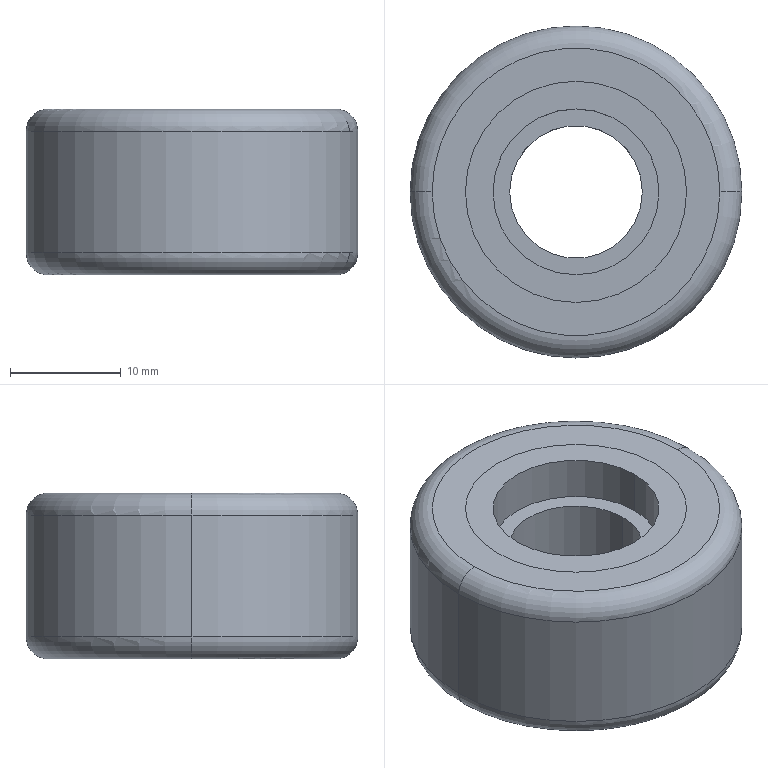Part | SolidWorks | features ICE 4, Extrusion 1, Fillet 1 | 2 solids | 22 faces | box 30 x 30 x 15 mm | volume 8240 mm3 | cylinder 12 | plane 6 | torus 4 | commonest cylinder face diameters 15 x4 20 x4 12 x2 30 x2
STEP:
#1=CARTESIAN_POINT('',(-15.,0.,13.));
#2=VERTEX_POINT('',#1);
#3=CARTESIAN_POINT('',(15.,0.,13.));
#4=VERTEX_POINT('',#3);
#5=CARTESIAN_POINT('',(0.,0.,13.));
#6=DIRECTION('',(0.,0.,-1.));
#7=DIRECTION('',(1.,0.,0.));
#8=AXIS2_PLACEMENT_3D('',#5,#6,#7);
#9=CIRCLE('',#8,15.);
#10=EDGE_CURVE('',#2,#4,#9,.T.);
#11=ORIENTED_EDGE('',*,*,#10,.F.);
#12=CARTESIAN_POINT('',(-13.,0.,15.));
#13=VERTEX_POINT('',#12);
#14=CARTESIAN_POINT('',(-13.,0.,13.));
#15=DIRECTION('',(0.,1.,0.));
#16=DIRECTION('',(-1.,0.,0.));
#17=AXIS2_PLACEMENT_3D('',#14,#15,#16);
#18=CIRCLE('',#17,2.);
#19=EDGE_CURVE('',#2,#13,#18,.T.);
#20=ORIENTED_EDGE('',*,*,#19,.T.);
#21=CARTESIAN_POINT('',(13.,0.,15.));
#22=VERTEX_POINT('',#21);
#23=CARTESIAN_POINT('',(0.,0.,15.));
#24=DIRECTION('',(0.,0.,1.));
#25=DIRECTION('',(1.,0.,0.));
#26=AXIS2_PLACEMENT_3D('',#23,#24,#25);
#27=CIRCLE('',#26,13.);
#28=EDGE_CURVE('',#22,#13,#27,.T.);
#29=ORIENTED_EDGE('',*,*,#28,.F.);
#30=CARTESIAN_POINT('',(13.,0.,13.));
#31=DIRECTION('',(0.,-1.,0.));
#32=DIRECTION('',(0.,0.,-1.));
#33=AXIS2_PLACEMENT_3D('',#30,#31,#32);
#34=CIRCLE('',#33,2.);
#35=EDGE_CURVE('',#4,#22,#34,.T.);
#36=ORIENTED_EDGE('',*,*,#35,.F.);
#37=EDGE_LOOP('',(#11,#20,#29,#36));
#38=FACE_OUTER_BOUND('',#37,.T.);
#39=CARTESIAN_POINT('',(0.,0.,13.));
#40=DIRECTION('',(0.,0.,1.));
#41=DIRECTION('',(1.,0.,0.));
#42=AXIS2_PLACEMENT_3D('',#39,#40,#41);
#43=TOROIDAL_SURFACE('',#42,13.,2.);
#44=ADVANCED_FACE('',(#38),#43,.T.);
#45=CARTESIAN_POINT('',(-13.,0.,0.));
#46=VERTEX_POINT('',#45);
#47=CARTESIAN_POINT('',(13.,0.,0.));
#48=VERTEX_POINT('',#47);
#49=CARTESIAN_POINT('',(0.,0.,0.));
#50=DIRECTION('',(0.,0.,-1.));
#51=DIRECTION('',(1.,0.,0.));
#52=AXIS2_PLACEMENT_3D('',#49,#50,#51);
#53=CIRCLE('',#52,13.);
#54=EDGE_CURVE('',#46,#48,#53,.T.);
#55=ORIENTED_EDGE('',*,*,#54,.F.);
#56=CARTESIAN_POINT('',(-15.,0.,2.));
#57=VERTEX_POINT('',#56);
#58=CARTESIAN_POINT('',(-13.,0.,2.));
#59=DIRECTION('',(0.,1.,0.));
#60=DIRECTION('',(-1.,0.,0.));
#61=AXIS2_PLACEMENT_3D('',#58,#59,#60);
#62=CIRCLE('',#61,2.);
#63=EDGE_CURVE('',#46,#57,#62,.T.);
#64=ORIENTED_EDGE('',*,*,#63,.T.);
#65=CARTESIAN_POINT('',(15.,0.,2.));
#66=VERTEX_POINT('',#65);
#67=CARTESIAN_POINT('',(0.,0.,2.));
#68=DIRECTION('',(0.,0.,1.));
#69=DIRECTION('',(1.,0.,0.));
#70=AXIS2_PLACEMENT_3D('',#67,#68,#69);
#71=CIRCLE('',#70,15.);
#72=EDGE_CURVE('',#66,#57,#71,.T.);
#73=ORIENTED_EDGE('',*,*,#72,.F.);
#74=CARTESIAN_POINT('',(13.,0.,2.));
#75=DIRECTION('',(0.,-1.,0.));
#76=DIRECTION('',(0.,0.,-1.));
#77=AXIS2_PLACEMENT_3D('',#74,#75,#76);
#78=CIRCLE('',#77,2.);
#79=EDGE_CURVE('',#48,#66,#78,.T.);
#80=ORIENTED_EDGE('',*,*,#79,.F.);
#81=EDGE_LOOP('',(#55,#64,#73,#80));
#82=FACE_OUTER_BOUND('',#81,.T.);
#83=CARTESIAN_POINT('',(0.,0.,2.));
#84=DIRECTION('',(0.,0.,1.));
#85=DIRECTION('',(1.,0.,0.));
#86=AXIS2_PLACEMENT_3D('',#83,#84,#85);
#87=TOROIDAL_SURFACE('',#86,13.,2.);
#88=ADVANCED_FACE('',(#82),#87,.T.);
#89=CARTESIAN_POINT('',(10.,0.,0.));
#90=VERTEX_POINT('',#89);
#91=CARTESIAN_POINT('',(-10.,0.,0.));
#92=VERTEX_POINT('',#91);
#93=CARTESIAN_POINT('',(0.,0.,0.));
#94=DIRECTION('',(0.,0.,-1.));
#95=DIRECTION('',(1.,0.,0.));
#96=AXIS2_PLACEMENT_3D('',#93,#94,#95);
#97=CIRCLE('',#96,10.);
#98=EDGE_CURVE('',#90,#92,#97,.T.);
#99=ORIENTED_EDGE('',*,*,#98,.T.);
#100=CARTESIAN_POINT('',(-10.,0.,15.));
#101=VERTEX_POINT('',#100);
#102=CARTESIAN_POINT('',(-10.,0.,-42.426));
#103=DIRECTION('',(0.,0.,1.));
#104=VECTOR('',#103,1000.);
#105=LINE('',#102,#104);
#106=EDGE_CURVE('',#92,#101,#105,.T.);
#107=ORIENTED_EDGE('',*,*,#106,.T.);
#108=CARTESIAN_POINT('',(10.,0.,15.));
#109=VERTEX_POINT('',#108);
#110=CARTESIAN_POINT('',(0.,0.,15.));
#111=DIRECTION('',(0.,0.,1.));
#112=DIRECTION('',(1.,0.,0.));
#113=AXIS2_PLACEMENT_3D('',#110,#111,#112);
#114=CIRCLE('',#113,10.);
#115=EDGE_CURVE('',#101,#109,#114,.T.);
#116=ORIENTED_EDGE('',*,*,#115,.T.);
#117=CARTESIAN_POINT('',(10.,0.,-42.426));
#118=DIRECTION('',(0.,0.,1.));
#119=VECTOR('',#118,1000.);
#120=LINE('',#117,#119);
#121=EDGE_CURVE('',#90,#109,#120,.T.);
#122=ORIENTED_EDGE('',*,*,#121,.F.);
#123=EDGE_LOOP('',(#99,#107,#116,#122));
#124=FACE_OUTER_BOUND('',#123,.T.);
#125=CARTESIAN_POINT('',(0.,0.,-42.426));
#126=DIRECTION('',(0.,0.,1.));
#127=DIRECTION('',(1.,0.,0.));
#128=AXIS2_PLACEMENT_3D('',#125,#126,#127);
#129=CYLINDRICAL_SURFACE('',#128,10.);
#130=ADVANCED_FACE('',(#124),#129,.F.);
#131=ORIENTED_EDGE('',*,*,#72,.T.);
#132=CARTESIAN_POINT('',(-15.,0.,-42.426));
#133=DIRECTION('',(0.,0.,1.));
#134=VECTOR('',#133,1000.);
#135=LINE('',#132,#134);
#136=EDGE_CURVE('',#57,#2,#135,.T.);
#137=ORIENTED_EDGE('',*,*,#136,.T.);
#138=ORIENTED_EDGE('',*,*,#10,.T.);
#139=CARTESIAN_POINT('',(15.,0.,-42.426));
#140=DIRECTION('',(0.,0.,1.));
#141=VECTOR('',#140,1000.);
#142=LINE('',#139,#141);
#143=EDGE_CURVE('',#66,#4,#142,.T.);
#144=ORIENTED_EDGE('',*,*,#143,.F.);
#145=EDGE_LOOP('',(#131,#137,#138,#144));
#146=FACE_OUTER_BOUND('',#145,.T.);
#147=CARTESIAN_POINT('',(0.,0.,-42.426));
#148=DIRECTION('',(0.,0.,1.));
#149=DIRECTION('',(1.,0.,0.));
#150=AXIS2_PLACEMENT_3D('',#147,#148,#149);
#151=CYLINDRICAL_SURFACE('',#150,15.);
#152=ADVANCED_FACE('',(#146),#151,.T.);
#153=ORIENTED_EDGE('',*,*,#136,.F.);
#154=CARTESIAN_POINT('',(0.,0.,2.));
#155=DIRECTION('',(0.,0.,1.));
#156=DIRECTION('',(1.,0.,0.));
#157=AXIS2_PLACEMENT_3D('',#154,#155,#156);
#158=CIRCLE('',#157,15.);
#159=EDGE_CURVE('',#57,#66,#158,.T.);
#160=ORIENTED_EDGE('',*,*,#159,.T.);
#161=ORIENTED_EDGE('',*,*,#143,.T.);
#162=CARTESIAN_POINT('',(0.,0.,13.));
#163=DIRECTION('',(0.,0.,-1.));
#164=DIRECTION('',(1.,0.,0.));
#165=AXIS2_PLACEMENT_3D('',#162,#163,#164);
#166=CIRCLE('',#165,15.);
#167=EDGE_CURVE('',#4,#2,#166,.T.);
#168=ORIENTED_EDGE('',*,*,#167,.T.);
#169=EDGE_LOOP('',(#153,#160,#161,#168));
#170=FACE_OUTER_BOUND('',#169,.T.);
#171=CARTESIAN_POINT('',(0.,0.,-42.426));
#172=DIRECTION('',(0.,0.,1.));
#173=DIRECTION('',(1.,0.,0.));
#174=AXIS2_PLACEMENT_3D('',#171,#172,#173);
#175=CYLINDRICAL_SURFACE('',#174,15.);
#176=ADVANCED_FACE('',(#170),#175,.T.);
#177=ORIENTED_EDGE('',*,*,#28,.T.);
#178=CARTESIAN_POINT('',(0.,0.,15.));
#179=DIRECTION('',(0.,0.,1.));
#180=DIRECTION('',(1.,0.,0.));
#181=AXIS2_PLACEMENT_3D('',#178,#179,#180);
#182=CIRCLE('',#181,13.);
#183=EDGE_CURVE('',#13,#22,#182,.T.);
#184=ORIENTED_EDGE('',*,*,#183,.T.);
#185=EDGE_LOOP('',(#177,#184));
#186=FACE_OUTER_BOUND('',#185,.T.);
#187=CARTESIAN_POINT('',(0.,0.,15.));
#188=DIRECTION('',(0.,0.,1.));
#189=DIRECTION('',(1.,0.,0.));
#190=AXIS2_PLACEMENT_3D('',#187,#188,#189);
#191=CIRCLE('',#190,10.);
#192=EDGE_CURVE('',#109,#101,#191,.T.);
#193=ORIENTED_EDGE('',*,*,#192,.F.);
#194=ORIENTED_EDGE('',*,*,#115,.F.);
#195=EDGE_LOOP('',(#193,#194));
#196=FACE_BOUND('',#195,.T.);
#197=CARTESIAN_POINT('',(0.,0.,15.));
#198=DIRECTION('',(0.,0.,1.));
#199=DIRECTION('',(1.,0.,0.));
#200=AXIS2_PLACEMENT_3D('',#197,#198,#199);
#201=PLANE('',#200);
#202=ADVANCED_FACE('',(#186,#196),#201,.T.);
#203=ORIENTED_EDGE('',*,*,#106,.F.);
#204=CARTESIAN_POINT('',(0.,0.,0.));
#205=DIRECTION('',(0.,0.,-1.));
#206=DIRECTION('',(1.,0.,0.));
#207=AXIS2_PLACEMENT_3D('',#204,#205,#206);
#208=CIRCLE('',#207,10.);
#209=EDGE_CURVE('',#92,#90,#208,.T.);
#210=ORIENTED_EDGE('',*,*,#209,.T.);
#211=ORIENTED_EDGE('',*,*,#121,.T.);
#212=ORIENTED_EDGE('',*,*,#192,.T.);
#213=EDGE_LOOP('',(#203,#210,#211,#212));
#214=FACE_OUTER_BOUND('',#213,.T.);
#215=CARTESIAN_POINT('',(0.,0.,-42.426));
#216=DIRECTION('',(0.,0.,1.));
#217=DIRECTION('',(1.,0.,0.));
#218=AXIS2_PLACEMENT_3D('',#215,#216,#217);
#219=CYLINDRICAL_SURFACE('',#218,10.);
#220=ADVANCED_FACE('',(#214),#219,.F.);
#221=CARTESIAN_POINT('',(0.,0.,0.));
#222=DIRECTION('',(0.,0.,-1.));
#223=DIRECTION('',(1.,0.,0.));
#224=AXIS2_PLACEMENT_3D('',#221,#222,#223);
#225=CIRCLE('',#224,13.);
#226=EDGE_CURVE('',#48,#46,#225,.T.);
#227=ORIENTED_EDGE('',*,*,#226,.T.);
#228=ORIENTED_EDGE('',*,*,#54,.T.);
#229=EDGE_LOOP('',(#227,#228));
#230=FACE_OUTER_BOUND('',#229,.T.);
#231=ORIENTED_EDGE('',*,*,#98,.F.);
#232=ORIENTED_EDGE('',*,*,#209,.F.);
#233=EDGE_LOOP('',(#231,#232));
#234=FACE_BOUND('',#233,.T.);
#235=CARTESIAN_POINT('',(0.,0.,0.));
#236=DIRECTION('',(0.,0.,1.));
#237=DIRECTION('',(1.,0.,0.));
#238=AXIS2_PLACEMENT_3D('',#235,#236,#237);
#239=PLANE('',#238);
#240=ADVANCED_FACE('',(#230,#234),#239,.F.);
#241=ORIENTED_EDGE('',*,*,#63,.F.);
#242=ORIENTED_EDGE('',*,*,#226,.F.);
#243=ORIENTED_EDGE('',*,*,#79,.T.);
#244=ORIENTED_EDGE('',*,*,#159,.F.);
#245=EDGE_LOOP('',(#241,#242,#243,#244));
#246=FACE_OUTER_BOUND('',#245,.T.);
#247=CARTESIAN_POINT('',(0.,0.,2.));
#248=DIRECTION('',(0.,0.,1.));
#249=DIRECTION('',(1.,0.,0.));
#250=AXIS2_PLACEMENT_3D('',#247,#248,#249);
#251=TOROIDAL_SURFACE('',#250,13.,2.);
#252=ADVANCED_FACE('',(#246),#251,.T.);
#253=ORIENTED_EDGE('',*,*,#19,.F.);
#254=ORIENTED_EDGE('',*,*,#167,.F.);
#255=ORIENTED_EDGE('',*,*,#35,.T.);
#256=ORIENTED_EDGE('',*,*,#183,.F.);
#257=EDGE_LOOP('',(#253,#254,#255,#256));
#258=FACE_OUTER_BOUND('',#257,.T.);
#259=CARTESIAN_POINT('',(0.,0.,13.));
#260=DIRECTION('',(0.,0.,1.));
#261=DIRECTION('',(1.,0.,0.));
#262=AXIS2_PLACEMENT_3D('',#259,#260,#261);
#263=TOROIDAL_SURFACE('',#262,13.,2.);
#264=ADVANCED_FACE('',(#258),#263,.T.);
#265=CLOSED_SHELL('',(#44,#88,#130,#152,#176,#202,#220,#240,#252,#264));
#266=MANIFOLD_SOLID_BREP('',#265);
#267=CARTESIAN_POINT('',(7.5,0.,4.));
#268=VERTEX_POINT('',#267);
#269=CARTESIAN_POINT('',(-7.5,0.,4.));
#270=VERTEX_POINT('',#269);
#271=CARTESIAN_POINT('',(0.,0.,4.));
#272=DIRECTION('',(0.,0.,-1.));
#273=DIRECTION('',(-1.,0.,0.));
#274=AXIS2_PLACEMENT_3D('',#271,#272,#273);
#275=CIRCLE('',#274,7.5);
#276=EDGE_CURVE('',#268,#270,#275,.T.);
#277=ORIENTED_EDGE('',*,*,#276,.F.);
#278=CARTESIAN_POINT('',(7.5,0.,0.));
#279=VERTEX_POINT('',#278);
#280=CARTESIAN_POINT('',(7.5,0.,4.));
#281=DIRECTION('',(0.,0.,-1.));
#282=VECTOR('',#281,1000.);
#283=LINE('',#280,#282);
#284=EDGE_CURVE('',#268,#279,#283,.T.);
#285=ORIENTED_EDGE('',*,*,#284,.T.);
#286=CARTESIAN_POINT('',(-7.5,0.,0.));
#287=VERTEX_POINT('',#286);
#288=CARTESIAN_POINT('',(0.,0.,0.));
#289=DIRECTION('',(0.,0.,-1.));
#290=DIRECTION('',(-1.,0.,0.));
#291=AXIS2_PLACEMENT_3D('',#288,#289,#290);
#292=CIRCLE('',#291,7.5);
#293=EDGE_CURVE('',#279,#287,#292,.T.);
#294=ORIENTED_EDGE('',*,*,#293,.T.);
#295=CARTESIAN_POINT('',(-7.5,0.,4.));
#296=DIRECTION('',(0.,0.,-1.));
#297=VECTOR('',#296,1000.);
#298=LINE('',#295,#297);
#299=EDGE_CURVE('',#270,#287,#298,.T.);
#300=ORIENTED_EDGE('',*,*,#299,.F.);
#301=EDGE_LOOP('',(#277,#285,#294,#300));
#302=FACE_OUTER_BOUND('',#301,.T.);
#303=CARTESIAN_POINT('',(0.,0.,4.));
#304=DIRECTION('',(0.,0.,-1.));
#305=DIRECTION('',(-1.,0.,0.));
#306=AXIS2_PLACEMENT_3D('',#303,#304,#305);
#307=CYLINDRICAL_SURFACE('',#306,7.5);
#308=ADVANCED_FACE('',(#302),#307,.F.);
#309=CARTESIAN_POINT('',(-7.5,0.,11.));
#310=VERTEX_POINT('',#309);
#311=CARTESIAN_POINT('',(7.5,0.,11.));
#312=VERTEX_POINT('',#311);
#313=CARTESIAN_POINT('',(0.,0.,11.));
#314=DIRECTION('',(0.,0.,1.));
#315=DIRECTION('',(1.,0.,0.));
#316=AXIS2_PLACEMENT_3D('',#313,#314,#315);
#317=CIRCLE('',#316,7.5);
#318=EDGE_CURVE('',#310,#312,#317,.T.);
#319=ORIENTED_EDGE('',*,*,#318,.F.);
#320=CARTESIAN_POINT('',(-7.5,0.,15.));
#321=VERTEX_POINT('',#320);
#322=CARTESIAN_POINT('',(-7.5,0.,11.));
#323=DIRECTION('',(0.,0.,1.));
#324=VECTOR('',#323,1000.);
#325=LINE('',#322,#324);
#326=EDGE_CURVE('',#310,#321,#325,.T.);
#327=ORIENTED_EDGE('',*,*,#326,.T.);
#328=CARTESIAN_POINT('',(7.5,0.,15.));
#329=VERTEX_POINT('',#328);
#330=CARTESIAN_POINT('',(0.,0.,15.));
#331=DIRECTION('',(0.,0.,1.));
#332=DIRECTION('',(1.,0.,0.));
#333=AXIS2_PLACEMENT_3D('',#330,#331,#332);
#334=CIRCLE('',#333,7.5);
#335=EDGE_CURVE('',#321,#329,#334,.T.);
#336=ORIENTED_EDGE('',*,*,#335,.T.);
#337=CARTESIAN_POINT('',(7.5,0.,11.));
#338=DIRECTION('',(0.,0.,1.));
#339=VECTOR('',#338,1000.);
#340=LINE('',#337,#339);
#341=EDGE_CURVE('',#312,#329,#340,.T.);
#342=ORIENTED_EDGE('',*,*,#341,.F.);
#343=EDGE_LOOP('',(#319,#327,#336,#342));
#344=FACE_OUTER_BOUND('',#343,.T.);
#345=CARTESIAN_POINT('',(0.,0.,11.));
#346=DIRECTION('',(0.,0.,1.));
#347=DIRECTION('',(1.,0.,0.));
#348=AXIS2_PLACEMENT_3D('',#345,#346,#347);
#349=CYLINDRICAL_SURFACE('',#348,7.5);
#350=ADVANCED_FACE('',(#344),#349,.F.);
#351=CARTESIAN_POINT('',(10.,0.,15.));
#352=VERTEX_POINT('',#351);
#353=CARTESIAN_POINT('',(-10.,0.,15.));
#354=VERTEX_POINT('',#353);
#355=CARTESIAN_POINT('',(0.,0.,15.));
#356=DIRECTION('',(0.,0.,1.));
#357=DIRECTION('',(1.,0.,0.));
#358=AXIS2_PLACEMENT_3D('',#355,#356,#357);
#359=CIRCLE('',#358,10.);
#360=EDGE_CURVE('',#352,#354,#359,.T.);
#361=ORIENTED_EDGE('',*,*,#360,.F.);
#362=CARTESIAN_POINT('',(10.,0.,0.));
#363=VERTEX_POINT('',#362);
#364=CARTESIAN_POINT('',(10.,0.,15.));
#365=DIRECTION('',(0.,0.,-1.));
#366=VECTOR('',#365,1000.);
#367=LINE('',#364,#366);
#368=EDGE_CURVE('',#352,#363,#367,.T.);
#369=ORIENTED_EDGE('',*,*,#368,.T.);
#370=CARTESIAN_POINT('',(-10.,0.,0.));
#371=VERTEX_POINT('',#370);
#372=CARTESIAN_POINT('',(0.,0.,0.));
#373=DIRECTION('',(0.,0.,1.));
#374=DIRECTION('',(1.,0.,0.));
#375=AXIS2_PLACEMENT_3D('',#372,#373,#374);
#376=CIRCLE('',#375,10.);
#377=EDGE_CURVE('',#363,#371,#376,.T.);
#378=ORIENTED_EDGE('',*,*,#377,.T.);
#379=CARTESIAN_POINT('',(-10.,0.,15.));
#380=DIRECTION('',(0.,0.,-1.));
#381=VECTOR('',#380,1000.);
#382=LINE('',#379,#381);
#383=EDGE_CURVE('',#354,#371,#382,.T.);
#384=ORIENTED_EDGE('',*,*,#383,.F.);
#385=EDGE_LOOP('',(#361,#369,#378,#384));
#386=FACE_OUTER_BOUND('',#385,.T.);
#387=CARTESIAN_POINT('',(0.,0.,15.));
#388=DIRECTION('',(0.,0.,-1.));
#389=DIRECTION('',(-1.,0.,0.));
#390=AXIS2_PLACEMENT_3D('',#387,#388,#389);
#391=CYLINDRICAL_SURFACE('',#390,10.);
#392=ADVANCED_FACE('',(#386),#391,.T.);
#393=CARTESIAN_POINT('',(-6.,0.,4.));
#394=VERTEX_POINT('',#393);
#395=CARTESIAN_POINT('',(6.,0.,4.));
#396=VERTEX_POINT('',#395);
#397=CARTESIAN_POINT('',(0.,0.,4.));
#398=DIRECTION('',(0.,0.,1.));
#399=DIRECTION('',(-1.,0.,0.));
#400=AXIS2_PLACEMENT_3D('',#397,#398,#399);
#401=CIRCLE('',#400,6.);
#402=EDGE_CURVE('',#394,#396,#401,.T.);
#403=ORIENTED_EDGE('',*,*,#402,.F.);
#404=CARTESIAN_POINT('',(-6.,0.,11.));
#405=VERTEX_POINT('',#404);
#406=CARTESIAN_POINT('',(-6.,0.,0.));
#407=DIRECTION('',(0.,0.,1.));
#408=VECTOR('',#407,1000.);
#409=LINE('',#406,#408);
#410=EDGE_CURVE('',#394,#405,#409,.T.);
#411=ORIENTED_EDGE('',*,*,#410,.T.);
#412=CARTESIAN_POINT('',(6.,0.,11.));
#413=VERTEX_POINT('',#412);
#414=CARTESIAN_POINT('',(0.,0.,11.));
#415=DIRECTION('',(0.,0.,-1.));
#416=DIRECTION('',(1.,0.,0.));
#417=AXIS2_PLACEMENT_3D('',#414,#415,#416);
#418=CIRCLE('',#417,6.);
#419=EDGE_CURVE('',#413,#405,#418,.T.);
#420=ORIENTED_EDGE('',*,*,#419,.F.);
#421=CARTESIAN_POINT('',(6.,0.,0.));
#422=DIRECTION('',(0.,0.,1.));
#423=VECTOR('',#422,1000.);
#424=LINE('',#421,#423);
#425=EDGE_CURVE('',#396,#413,#424,.T.);
#426=ORIENTED_EDGE('',*,*,#425,.F.);
#427=EDGE_LOOP('',(#403,#411,#420,#426));
#428=FACE_OUTER_BOUND('',#427,.T.);
#429=CARTESIAN_POINT('',(0.,0.,0.));
#430=DIRECTION('',(0.,0.,1.));
#431=DIRECTION('',(1.,0.,0.));
#432=AXIS2_PLACEMENT_3D('',#429,#430,#431);
#433=CYLINDRICAL_SURFACE('',#432,6.);
#434=ADVANCED_FACE('',(#428),#433,.F.);
#435=ORIENTED_EDGE('',*,*,#410,.F.);
#436=CARTESIAN_POINT('',(0.,0.,4.));
#437=DIRECTION('',(0.,0.,1.));
#438=DIRECTION('',(-1.,0.,0.));
#439=AXIS2_PLACEMENT_3D('',#436,#437,#438);
#440=CIRCLE('',#439,6.);
#441=EDGE_CURVE('',#396,#394,#440,.T.);
#442=ORIENTED_EDGE('',*,*,#441,.F.);
#443=ORIENTED_EDGE('',*,*,#425,.T.);
#444=CARTESIAN_POINT('',(0.,0.,11.));
#445=DIRECTION('',(0.,0.,-1.));
#446=DIRECTION('',(1.,0.,0.));
#447=AXIS2_PLACEMENT_3D('',#444,#445,#446);
#448=CIRCLE('',#447,6.);
#449=EDGE_CURVE('',#405,#413,#448,.T.);
#450=ORIENTED_EDGE('',*,*,#449,.F.);
#451=EDGE_LOOP('',(#435,#442,#443,#450));
#452=FACE_OUTER_BOUND('',#451,.T.);
#453=CARTESIAN_POINT('',(0.,0.,0.));
#454=DIRECTION('',(0.,0.,1.));
#455=DIRECTION('',(1.,0.,0.));
#456=AXIS2_PLACEMENT_3D('',#453,#454,#455);
#457=CYLINDRICAL_SURFACE('',#456,6.);
#458=ADVANCED_FACE('',(#452),#457,.F.);
#459=ORIENTED_EDGE('',*,*,#368,.F.);
#460=CARTESIAN_POINT('',(0.,0.,15.));
#461=DIRECTION('',(0.,0.,1.));
#462=DIRECTION('',(1.,0.,0.));
#463=AXIS2_PLACEMENT_3D('',#460,#461,#462);
#464=CIRCLE('',#463,10.);
#465=EDGE_CURVE('',#354,#352,#464,.T.);
#466=ORIENTED_EDGE('',*,*,#465,.F.);
#467=ORIENTED_EDGE('',*,*,#383,.T.);
#468=CARTESIAN_POINT('',(0.,0.,0.));
#469=DIRECTION('',(0.,0.,1.));
#470=DIRECTION('',(1.,0.,0.));
#471=AXIS2_PLACEMENT_3D('',#468,#469,#470);
#472=CIRCLE('',#471,10.);
#473=EDGE_CURVE('',#371,#363,#472,.T.);
#474=ORIENTED_EDGE('',*,*,#473,.T.);
#475=EDGE_LOOP('',(#459,#466,#467,#474));
#476=FACE_OUTER_BOUND('',#475,.T.);
#477=CARTESIAN_POINT('',(0.,0.,15.));
#478=DIRECTION('',(0.,0.,-1.));
#479=DIRECTION('',(-1.,0.,0.));
#480=AXIS2_PLACEMENT_3D('',#477,#478,#479);
#481=CYLINDRICAL_SURFACE('',#480,10.);
#482=ADVANCED_FACE('',(#476),#481,.T.);
#483=CARTESIAN_POINT('',(0.,0.,15.));
#484=DIRECTION('',(0.,0.,1.));
#485=DIRECTION('',(1.,0.,0.));
#486=AXIS2_PLACEMENT_3D('',#483,#484,#485);
#487=CIRCLE('',#486,7.5);
#488=EDGE_CURVE('',#329,#321,#487,.T.);
#489=ORIENTED_EDGE('',*,*,#488,.F.);
#490=ORIENTED_EDGE('',*,*,#335,.F.);
#491=EDGE_LOOP('',(#489,#490));
#492=FACE_BOUND('',#491,.T.);
#493=ORIENTED_EDGE('',*,*,#465,.T.);
#494=ORIENTED_EDGE('',*,*,#360,.T.);
#495=EDGE_LOOP('',(#493,#494));
#496=FACE_OUTER_BOUND('',#495,.T.);
#497=CARTESIAN_POINT('',(0.,0.,15.));
#498=DIRECTION('',(0.,0.,1.));
#499=DIRECTION('',(1.,0.,0.));
#500=AXIS2_PLACEMENT_3D('',#497,#498,#499);
#501=PLANE('',#500);
#502=ADVANCED_FACE('',(#492,#496),#501,.T.);
#503=CARTESIAN_POINT('',(0.,0.,0.));
#504=DIRECTION('',(0.,0.,-1.));
#505=DIRECTION('',(-1.,0.,0.));
#506=AXIS2_PLACEMENT_3D('',#503,#504,#505);
#507=CIRCLE('',#506,7.5);
#508=EDGE_CURVE('',#287,#279,#507,.T.);
#509=ORIENTED_EDGE('',*,*,#508,.F.);
#510=ORIENTED_EDGE('',*,*,#293,.F.);
#511=EDGE_LOOP('',(#509,#510));
#512=FACE_BOUND('',#511,.T.);
#513=ORIENTED_EDGE('',*,*,#473,.F.);
#514=ORIENTED_EDGE('',*,*,#377,.F.);
#515=EDGE_LOOP('',(#513,#514));
#516=FACE_OUTER_BOUND('',#515,.T.);
#517=CARTESIAN_POINT('',(0.,0.,0.));
#518=DIRECTION('',(0.,0.,1.));
#519=DIRECTION('',(1.,0.,0.));
#520=AXIS2_PLACEMENT_3D('',#517,#518,#519);
#521=PLANE('',#520);
#522=ADVANCED_FACE('',(#512,#516),#521,.F.);
#523=CARTESIAN_POINT('',(0.,0.,11.));
#524=DIRECTION('',(0.,0.,1.));
#525=DIRECTION('',(1.,0.,0.));
#526=AXIS2_PLACEMENT_3D('',#523,#524,#525);
#527=CIRCLE('',#526,7.5);
#528=EDGE_CURVE('',#312,#310,#527,.T.);
#529=ORIENTED_EDGE('',*,*,#528,.T.);
#530=ORIENTED_EDGE('',*,*,#318,.T.);
#531=EDGE_LOOP('',(#529,#530));
#532=FACE_OUTER_BOUND('',#531,.T.);
#533=ORIENTED_EDGE('',*,*,#419,.T.);
#534=ORIENTED_EDGE('',*,*,#449,.T.);
#535=EDGE_LOOP('',(#533,#534));
#536=FACE_BOUND('',#535,.T.);
#537=CARTESIAN_POINT('',(0.,0.,11.));
#538=DIRECTION('',(0.,0.,1.));
#539=DIRECTION('',(1.,0.,0.));
#540=AXIS2_PLACEMENT_3D('',#537,#538,#539);
#541=PLANE('',#540);
#542=ADVANCED_FACE('',(#532,#536),#541,.T.);
#543=ORIENTED_EDGE('',*,*,#326,.F.);
#544=ORIENTED_EDGE('',*,*,#528,.F.);
#545=ORIENTED_EDGE('',*,*,#341,.T.);
#546=ORIENTED_EDGE('',*,*,#488,.T.);
#547=EDGE_LOOP('',(#543,#544,#545,#546));
#548=FACE_OUTER_BOUND('',#547,.T.);
#549=CARTESIAN_POINT('',(0.,0.,11.));
#550=DIRECTION('',(0.,0.,1.));
#551=DIRECTION('',(1.,0.,0.));
#552=AXIS2_PLACEMENT_3D('',#549,#550,#551);
#553=CYLINDRICAL_SURFACE('',#552,7.5);
#554=ADVANCED_FACE('',(#548),#553,.F.);
#555=CARTESIAN_POINT('',(0.,0.,4.));
#556=DIRECTION('',(0.,0.,-1.));
#557=DIRECTION('',(-1.,0.,0.));
#558=AXIS2_PLACEMENT_3D('',#555,#556,#557);
#559=CIRCLE('',#558,7.5);
#560=EDGE_CURVE('',#270,#268,#559,.T.);
#561=ORIENTED_EDGE('',*,*,#560,.T.);
#562=ORIENTED_EDGE('',*,*,#276,.T.);
#563=EDGE_LOOP('',(#561,#562));
#564=FACE_OUTER_BOUND('',#563,.T.);
#565=ORIENTED_EDGE('',*,*,#441,.T.);
#566=ORIENTED_EDGE('',*,*,#402,.T.);
#567=EDGE_LOOP('',(#565,#566));
#568=FACE_BOUND('',#567,.T.);
#569=CARTESIAN_POINT('',(0.,0.,4.));
#570=DIRECTION('',(0.,0.,-1.));
#571=DIRECTION('',(-1.,0.,0.));
#572=AXIS2_PLACEMENT_3D('',#569,#570,#571);
#573=PLANE('',#572);
#574=ADVANCED_FACE('',(#564,#568),#573,.T.);
#575=ORIENTED_EDGE('',*,*,#284,.F.);
#576=ORIENTED_EDGE('',*,*,#560,.F.);
#577=ORIENTED_EDGE('',*,*,#299,.T.);
#578=ORIENTED_EDGE('',*,*,#508,.T.);
#579=EDGE_LOOP('',(#575,#576,#577,#578));
#580=FACE_OUTER_BOUND('',#579,.T.);
#581=CARTESIAN_POINT('',(0.,0.,4.));
#582=DIRECTION('',(0.,0.,-1.));
#583=DIRECTION('',(-1.,0.,0.));
#584=AXIS2_PLACEMENT_3D('',#581,#582,#583);
#585=CYLINDRICAL_SURFACE('',#584,7.5);
#586=ADVANCED_FACE('',(#580),#585,.F.);
#587=CLOSED_SHELL('',(#308,#350,#392,#434,#458,#482,#502,#522,#542,#554,#574,#586));
#588=MANIFOLD_SOLID_BREP('',#587);
#589=CARTESIAN_POINT('',(0.,0.,0.));
#590=DIRECTION('',(0.,0.,1.));
#591=DIRECTION('',(1.,0.,0.));
#592=AXIS2_PLACEMENT_3D('',#589,#590,#591);
#593=(LENGTH_UNIT()NAMED_UNIT(*)SI_UNIT(.MILLI.,.METRE.));
#594=UNCERTAINTY_MEASURE_WITH_UNIT(LENGTH_MEASURE(0.00001),#593,'','');
#595=(NAMED_UNIT(*)PLANE_ANGLE_UNIT()SI_UNIT($,.RADIAN.));
#596=(NAMED_UNIT(*)SI_UNIT($,.STERADIAN.)SOLID_ANGLE_UNIT());
#597=(GEOMETRIC_REPRESENTATION_CONTEXT(3)GLOBAL_UNCERTAINTY_ASSIGNED_CONTEXT((#594))GLOBAL_UNIT_ASSIGNED_CONTEXT((#593,#595,#596))REPRESENTATION_CONTEXT('',''));
#598=ADVANCED_BREP_SHAPE_REPRESENTATION('',(#266,#588,#592),#597);